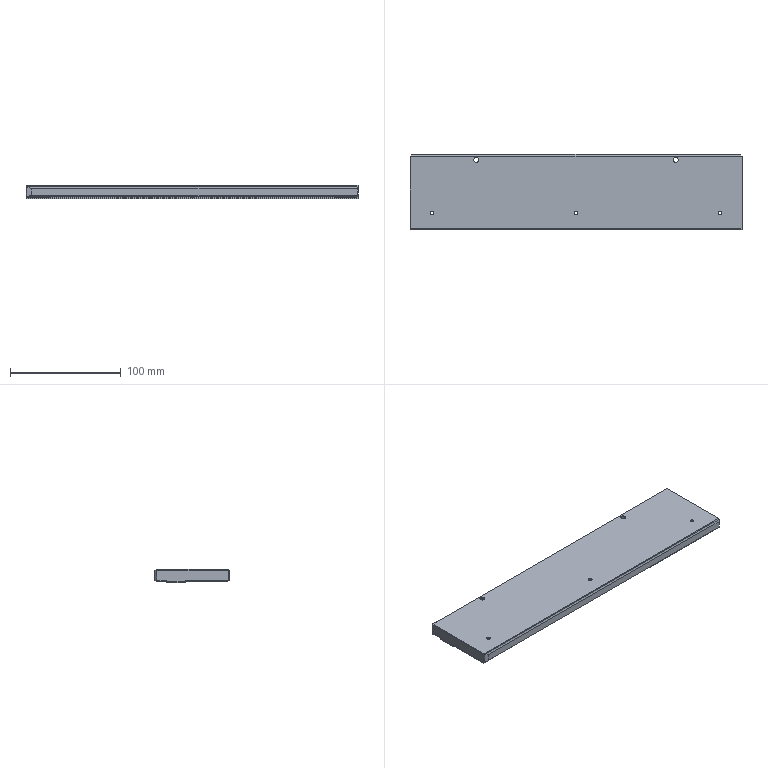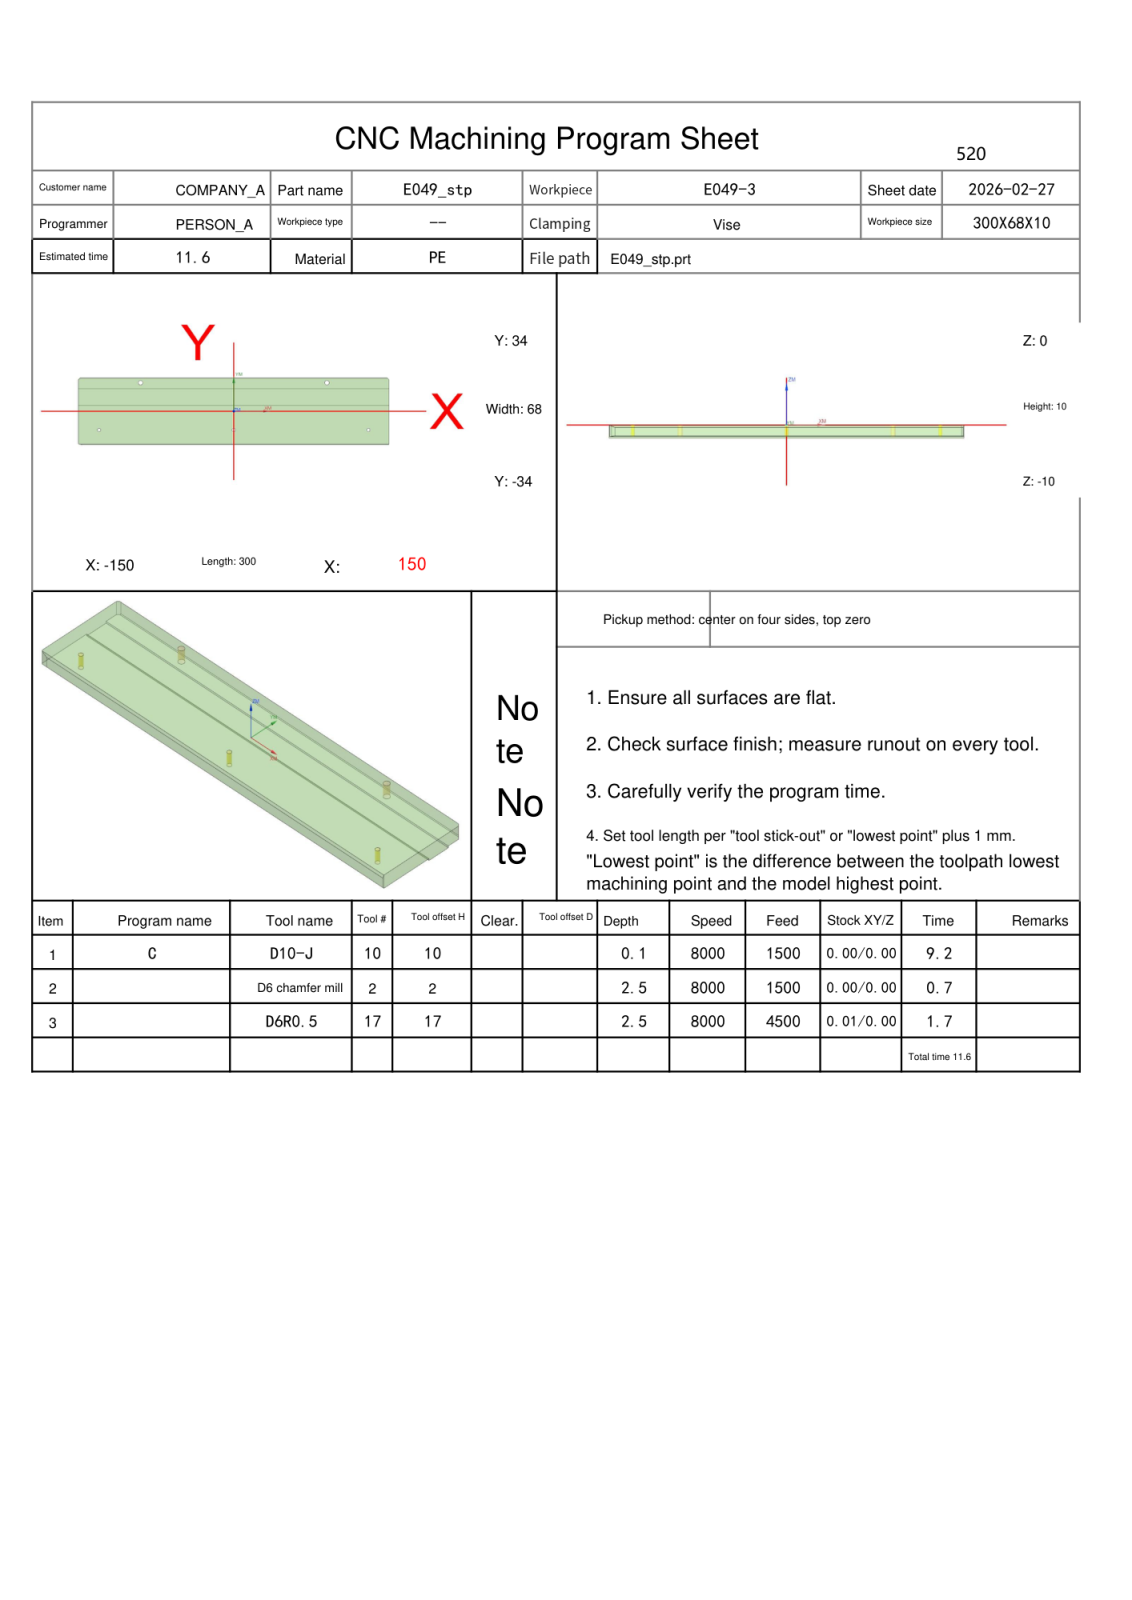NC program | NX | posted by the shop | part box 300 x 68 x 12 mm
Whole program:
%
O0001
(Machine time: 12.22 MIN)
(===Total Tool:3===)
(T10=D10-J  D=10.  R=0.   D-  H10 Z=-0.   )
(T2=D6 chamfer mill   D=6.   R=0.   D-  H02 Z=-2.55 )
(T17=D6R0.5 D=6.   R=0.5  D-  H17 Z=-2.5  )
G80 G90 G17 G49 G40
G91 G28 Z0
M01
N1 T10 M06
(D10-J  D=10. R=0. H=10 ce=0.00 di=0.10)
G00 G90 G54 X-160. Y24.3 M03 S4500
G43 H10 Z30.
M08
Z2.55
G01 Z.55 F1500.
X-155. Y29.3
X-145.3 Y39.
X-135.6
X-155. Y19.6
Y9.9
X-125.9 Y39.
X-116.2
X-155. Y.2
Y-9.5
X-106.5 Y39.
X-96.8
X-155. Y-19.2
Y-28.9
X-87.1 Y39.
X-77.4
X-155. Y-38.6
Y-39.
X-145.7
X-67.7 Y39.
X-58.
X-136. Y-39.
X-126.3
X-48.3 Y39.
X-38.6
X-116.6 Y-39.
X-106.9
X-28.9 Y39.
X-19.2
X-97.2 Y-39.
X-87.5
X-9.5 Y39.
X.2
X-77.8 Y-39.
X-68.1
X9.9 Y39.
X19.6
X-58.4 Y-39.
X-48.7
X29.3 Y39.
X39.
X-39. Y-39.
X-29.3
X48.7 Y39.
X58.4
X-19.6 Y-39.
X-9.9
X68.1 Y39.
X77.8
X-.2 Y-39.
X9.5
X87.5 Y39.
X97.2
X19.2 Y-39.
X28.9
X106.9 Y39.
X116.6
X38.6 Y-39.
X48.3
X126.3 Y39.
X136.
X58. Y-39.
X67.7
X145.7 Y39.
X155.
Y38.6
X77.4 Y-39.
X87.1
X155. Y28.9
Y19.2
X96.8 Y-39.
X106.5
X155. Y9.5
Y-.2
X116.2 Y-39.
X125.9
X155. Y-9.9
Y-19.6
X135.6 Y-39.
X145.3
X155. Y-29.3
X160. Y-24.3
Z2.55
G00 Z4.
X-160. Y24.3
Z2.1
G01 Z.1
X-155. Y29.3
X-145.3 Y39.
X-135.6
X-155. Y19.6
Y9.9
X-125.9 Y39.
X-116.2
X-155. Y.2
Y-9.5
X-106.5 Y39.
X-96.8
X-155. Y-19.2
Y-28.9
X-87.1 Y39.
X-77.4
X-155. Y-38.6
Y-39.
X-145.7
X-67.7 Y39.
X-58.
X-136. Y-39.
X-126.3
X-48.3 Y39.
X-38.6
X-116.6 Y-39.
X-106.9
X-28.9 Y39.
X-19.2
X-97.2 Y-39.
X-87.5
X-9.5 Y39.
X.2
X-77.8 Y-39.
X-68.1
X9.9 Y39.
X19.6
X-58.4 Y-39.
X-48.7
X29.3 Y39.
X39.
X-39. Y-39.
X-29.3
X48.7 Y39.
X58.4
X-19.6 Y-39.
X-9.9
X68.1 Y39.
X77.8
X-.2 Y-39.
X9.5
X87.5 Y39.
X97.2
X19.2 Y-39.
X28.9
X106.9 Y39.
X116.6
X38.6 Y-39.
X48.3
X126.3 Y39.
X136.
X58. Y-39.
X67.7
X145.7 Y39.
X155.
Y38.6
X77.4 Y-39.
X87.1
X155. Y28.9
Y19.2
X96.8 Y-39.
X106.5
X155. Y9.5
Y-.2
X116.2 Y-39.
X125.9
X155. Y-9.9
Y-19.6
X135.6 Y-39.
X145.3
X155. Y-29.3
X160. Y-24.3
Z2.1
G00 Z30.
G00 G90 X133.3 Y51. M03 S8000
Z30.
Z2.
G01 Z0.0 F1000.
X145.3 Y39.
X155. Y29.3
Y19.6
X135.6 Y39.
X125.9
X155. Y9.9
Y.2
X116.2 Y39.
X106.5
X155. Y-9.5
Y-19.2
X96.8 Y39.
X87.1
X155. Y-28.9
Y-38.6
X77.4 Y39.
X67.7
X145.7 Y-39.
X136.
X58. Y39.
X48.3
X126.3 Y-39.
X116.6
X38.6 Y39.
X28.9
X106.9 Y-39.
X97.2
X19.2 Y39.
X9.5
X87.5 Y-39.
X77.8
X-.2 Y39.
X-9.9
X68.1 Y-39.
X58.4
X-19.6 Y39.
X-29.3
X48.7 Y-39.
X39.
X-39. Y39.
X-48.7
X29.3 Y-39.
X19.6
X-58.4 Y39.
X-68.1
X9.9 Y-39.
X.2
X-77.8 Y39.
X-87.5
X-9.5 Y-39.
X-19.2
X-97.2 Y39.
X-106.9
X-28.9 Y-39.
X-38.6
X-116.6 Y39.
X-126.3
X-48.3 Y-39.
X-58.
X-136. Y39.
X-145.7
X-67.7 Y-39.
X-77.4
X-155. Y38.6
Y28.9
X-87.1 Y-39.
X-96.8
X-155. Y19.2
Y9.5
X-106.5 Y-39.
X-116.2
X-155. Y-.2
Y-9.9
X-125.9 Y-39.
X-135.6
X-155. Y-19.6
Y-29.3
X-145.3 Y-39.
X-133.3 Y-51.
Z2.
G00 Z30.
G91 G28 Z0.0
M05
M09
G91 G28 Z0.0
M01
N2 T02 M06
(D6 chamfer mill  D=6. R=0. H=02 ce=0.00 di=0.00)
G00 G90 G54 X130. Y-19. M03 S8000
G43 H02 Z30.
M08
G98 G81 X130. Y-19. Z-1.921 R3. F1000.
X0.0
X-130.
G80
G00 Z30.
G00 G90 X-90. Y29. M03 S8000
Z30.
G98 G81 X-90. Y29. Z-2.55 R3. F1000.
X90.
G80
G00 Z30.
G00 G90 X148.91 Y34.403 M03 S6500
Z30.
Z2.8
G01 Z-1.2 F1500.
X149. Y34.366
X149.207 Y34.207
X150.707 Y32.707
X150.866 Y32.5
X150.966 Y32.259
X151. Y32.
Y-33.5
G02 X150. Y-34.5 I-1. J0.0
G01 X.226
X-149.548
X-149.822 Y-34.461
X-150.076 Y-34.349
X-150.289 Y-34.171
X-150.741 Y-33.671
X-150.882 Y-33.471
X-150.97 Y-33.243
X-151. Y-33.
Y32.
X-150.966 Y32.259
X-150.866 Y32.5
X-150.707 Y32.707
X-149.207 Y34.207
X-149. Y34.366
X-148.91 Y34.403
Z2.8
G00 Z10.
X-129.535 Y-19.419
Z.413
G01 Z-1.2
G03 X-129.388 Y-19.103 I-1.732 J1.
G01 X-129.367 Y-19.053
X-129.379 Y-19.
G03 X-130. Y-18.379 I-.621 J0.0
X-130.621 Y-19. I0.0 J-.621
X-130. Y-19.621 I.621 J0.0
X-129.379 Y-19. I0.0 J.621
G01 X-129.367 Y-18.947
X-129.388 Y-18.897
G03 X-129.535 Y-18.581 I-1.879 J-.684
G01 Z.413
G00 Z10.
X-88.935 Y28.593
Z.294
G01 Z-1.2
G03 X-88.766 Y28.898 I-1.658 J1.118
G01 X-88.741 Y28.946
X-88.75 Y29.
G03 X-90. Y30.25 I-1.25 J0.0
X-91.25 Y29. I0.0 J-1.25
X-90. Y27.75 I1.25 J0.0
X-88.777 Y28.74 I0.0 J1.25
G01 X-88.75 Y29.
X-88.741 Y29.054
X-88.766 Y29.102
G03 X-88.935 Y29.407 I-1.827 J-.813
G01 Z.294
G00 Z10.
X.465 Y-19.419
Z.413
G01 Z-1.2
G03 X.612 Y-19.103 I-1.732 J1.
G01 X.633 Y-19.053
X.621 Y-19.
G03 X0.0 Y-18.379 I-.621 J0.0
X-.621 Y-19. I0.0 J-.621
X0.0 Y-19.621 I.621 J0.0
X.621 Y-19. I0.0 J.621
G01 X.633 Y-18.947
X.612 Y-18.897
G03 X.465 Y-18.581 I-1.879 J-.684
G01 Z.413
G00 Z10.
X91.065 Y28.593
Z.294
G01 Z-1.2
G03 X91.234 Y28.898 I-1.658 J1.118
G01 X91.259 Y28.946
X91.25 Y29.
G03 X90. Y30.25 I-1.25 J0.0
X88.75 Y29. I0.0 J-1.25
X90. Y27.75 I1.25 J0.0
X91.223 Y28.74 I0.0 J1.25
G01 X91.25 Y29.
X91.259 Y29.054
X91.234 Y29.102
G03 X91.065 Y29.407 I-1.827 J-.813
G01 Z.294
G00 Z10.
X130.465 Y-19.419
Z.413
G01 Z-1.2
G03 X130.612 Y-19.103 I-1.732 J1.
G01 X130.633 Y-19.053
X130.621 Y-19.
G03 X130. Y-18.379 I-.621 J0.0
X129.379 Y-19. I0.0 J-.621
X130. Y-19.621 I.621 J0.0
X130.621 Y-19. I0.0 J.621
G01 X130.633 Y-18.947
X130.612 Y-18.897
G03 X130.465 Y-18.581 I-1.879 J-.684
G01 Z.413
G00 Z30.
G00 G90 X-152.407 Y35.9 M03 S6500
Z30.
Z.3
G01 Z-1.2 F1500.
G03 X-151.207 Y34.7 I1.2 J0.0
G01 X151.207
G03 X152.407 Y35.9 I0.0 J1.2
G01 Z.3
G00 Z30.
G91 G28 Z0.0
M05
M09
G91 G28 Z0.0
M01
N3 T17 M06
(D6R0.5  D=6. R=0.5 H=17 ce=0.01 di=0.00)
G00 G90 G54 X156.464 Y-36.422 M03 S8000
G43 H17 Z11.077
M08
Z.403
G01 Z-.097 F4500.
X151.152
X-150.704 Y-36.425
X-150.684 Y-36.449 Z-.194
X151.151 Y-36.446
X151.127 Y-36.47 Z-.291
X-150.657 Y-36.472
X-150.63 Y-36.496 Z-.388
X-150.357 Y-36.497
X151.051
X151.103 Y-36.495
X151.078 Y-36.52 Z-.485
X151.051 Y-36.522
X-150.357
X-150.602 Y-36.52
X-150.575 Y-36.544 Z-.582
X-150.357 Y-36.546
X149.949
X151.054
X151.03 Y-36.569 Z-.679
X149.925 Y-36.57
X-150.357
X-150.547 Y-36.568
X-150.52 Y-36.593 Z-.776
X-150.357 Y-36.594
X149.901
X151.005 Y-36.593
X150.981 Y-36.616 Z-.873
X149.876 Y-36.619
X-150.357
X-150.492 Y-36.617
X-150.465 Y-36.641 Z-.97
X-150.357 Y-36.643
X149.852
X150.956 Y-36.64
X150.932 Y-36.664 Z-1.067
X150.01 Y-36.667
X-150.357
X-150.437 Y-36.665
X-150.41 Y-36.69 Z-1.164
X-150.357 Y-36.691
X150.704
X150.908 Y-36.688
X150.883 Y-36.712 Z-1.261
X150.704 Y-36.716
X-150.357
X-150.383 Y-36.715
X-150.342 Y-36.739 Z-1.358
X-147.551 Y-36.74
X150.704
X150.859 Y-36.736
X150.834 Y-36.761 Z-1.455
X150.704 Y-36.764
X-150.01
X-150.101 Y-36.761
X-149.982 Y-36.776 Z-1.504
X-149.862 Y-36.787 Z-1.552
X-149.663 Y-36.788
X150.704
X150.81 Y-36.787
X150.786 Y-36.81 Z-1.649
X150.704 Y-36.813
X-149.316
X-149.621 Y-36.811
X-149.501 Y-36.825 Z-1.698
X-149.381 Y-36.835 Z-1.746
X-149.316 Y-36.837
X150.704
X150.761 Y-36.834
X150.737 Y-36.86 Z-1.843
X150.704 Y-36.861
X-148.969
X-149.141 Y-36.858
X-149.022 Y-36.873 Z-1.892
X-148.902 Y-36.883 Z-1.94
X-148.623 Y-36.885
X149.61
X150.712
X150.688 Y-36.909 Z-2.037
X149.585 Y-36.91
X-148.623
X-148.661 Y-36.908
X-148.54 Y-36.922 Z-2.086
X-148.42 Y-36.93 Z-2.134
X-148.276 Y-36.934
X149.561
X150.663 Y-36.932
X150.64 Y-36.955 Z-2.226
X149.538 Y-36.957
X-147.929
X-148.192 Y-36.954
X-148.078 Y-36.968 Z-2.271
X-147.963 Y-36.978 Z-2.317
X-147.929 Y-36.98
X149.515
X150.617 Y-36.977
X150.594 Y-36.999 Z-2.409
X-147.735
X-147.62 Y-37.014 Z-2.454
X-147.506 Y-37.023 Z-2.5
X150.571 Y-37.022
G00 Z11.077
M05
M09
G91 G28 Z0.0
G91 G28 Y0.0
M30
%